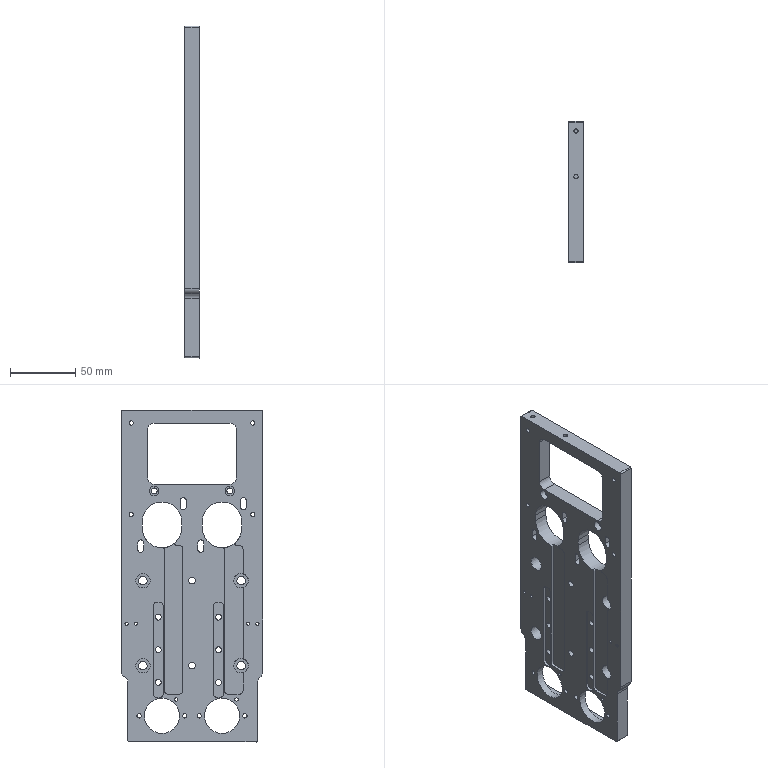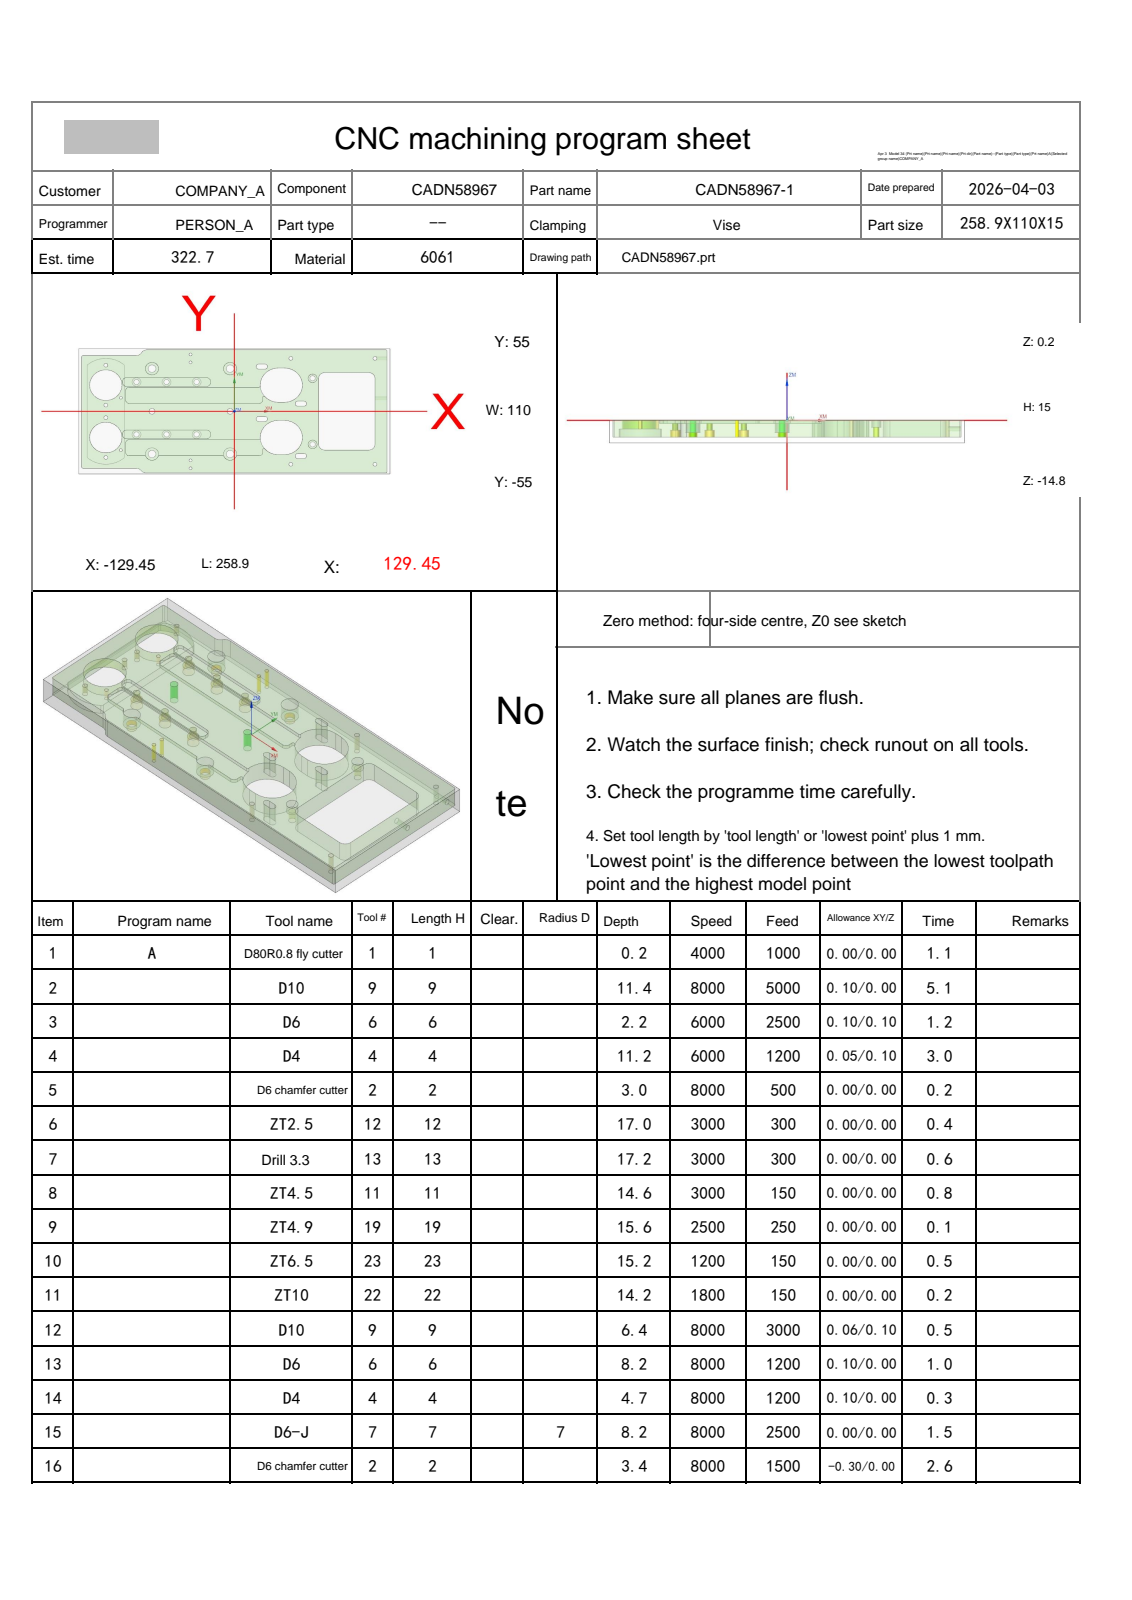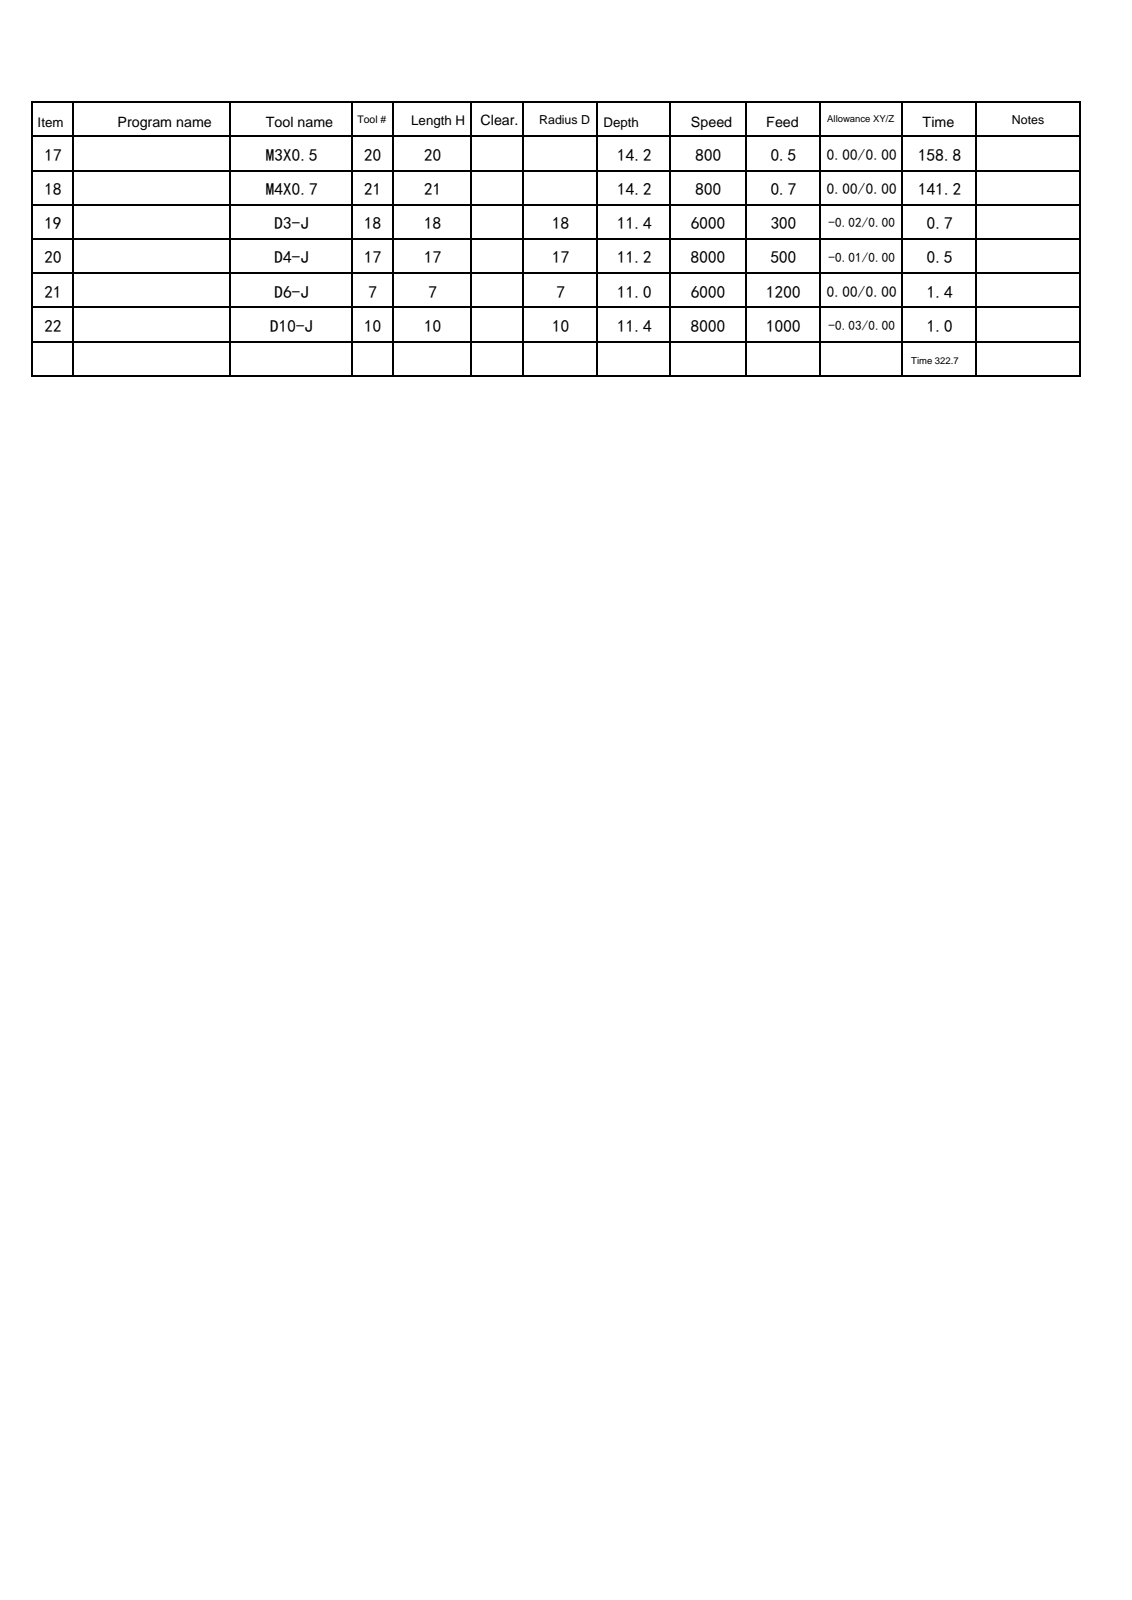NC program | NX | posted by the shop | part box 11 x 108 x 253.9 mm
Lines 911 to 1909 of 8037:
N4 T04 M06
(D4  D=4. R=0. H=04 ce=0.05 di=0.10)
G00 G90 G54 X22.813 Y39.463 M03 S6000
G43 H04 Z20.
M08
Z.5
G01 X20.313 Z.467 F1200.
G03 X20.113 Y39.263 Z.463 I0.0 J-.2
X20.313 Y39.063 Z.458 I.2 J0.0
G01 X25.313 Z.392
X25.376 Z.391
X25.434 Y39.091
X25.472 Y39.141 Z.39
X25.504 Y39.174 Z.389
X25.518 Y39.218
X25.513 Y39.263 Z.388
G03 X25.313 Y39.463 Z.384 I-.2 J0.0
G01 X20.313 Z.317
G03 X20.113 Y39.263 Z.313 I0.0 J-.2
X20.313 Y39.063 Z.309 I.2 J0.0
G01 X25.313 Z.243
X25.376 Z.242
X25.434 Y39.091 Z.241
X25.472 Y39.141 Z.24
X25.504 Y39.174
X25.518 Y39.218 Z.239
X25.513 Y39.263
G03 X25.313 Y39.463 Z.234 I-.2 J0.0
G01 X20.313 Z.168
G03 X20.113 Y39.263 Z.164 I0.0 J-.2
X20.313 Y39.063 Z.16 I.2 J0.0
G01 X25.313 Z.093
X25.376
X25.434 Y39.091 Z.092
X25.472 Y39.141 Z.091
X25.504 Y39.174 Z.09
X25.518 Y39.218
X25.513 Y39.263 Z.089
G03 X25.313 Y39.463 Z.085 I-.2 J0.0
G01 X20.313 Z.019
G03 X20.113 Y39.263 Z.015 I0.0 J-.2
X20.313 Y39.063 Z.01 I.2 J0.0
G01 X25.313 Z-.056
X25.376 Z-.057
X25.434 Y39.091 Z-.058
X25.472 Y39.141
X25.504 Y39.174 Z-.059
X25.518 Y39.218
X25.513 Y39.263 Z-.06
G03 X25.313 Y39.463 Z-.064 I-.2 J0.0
G01 X20.313 Z-.131
G03 X20.113 Y39.263 Z-.135 I0.0 J-.2
X20.313 Y39.063 Z-.139 I.2 J0.0
G01 X25.313 Z-.205
X25.376 Z-.206
X25.434 Y39.091 Z-.207
X25.472 Y39.141 Z-.208
X25.504 Y39.174
X25.518 Y39.218 Z-.209
X25.513 Y39.263
G03 X25.313 Y39.463 Z-.214 I-.2 J0.0
G01 X20.313 Z-.28
G03 X20.113 Y39.263 Z-.284 I0.0 J-.2
X20.313 Y39.063 Z-.288 I.2 J0.0
G01 X25.313 Z-.355
X25.376
X25.434 Y39.091 Z-.356
X25.472 Y39.141 Z-.357
X25.504 Y39.174 Z-.358
X25.518 Y39.218
X25.513 Y39.263 Z-.359
G03 X25.313 Y39.463 Z-.363 I-.2 J0.0
G01 X20.313 Z-.429
G03 X20.113 Y39.263 Z-.433 I0.0 J-.2
X20.313 Y39.063 Z-.438 I.2 J0.0
G01 X25.313 Z-.504
X25.376 Z-.505
X25.434 Y39.091 Z-.506
X25.472 Y39.141
X25.504 Y39.174 Z-.507
X25.518 Y39.218 Z-.508
X25.513 Y39.263
G03 X25.313 Y39.463 Z-.512 I-.2 J0.0
G01 X20.313 Z-.579
G03 X20.113 Y39.263 Z-.583 I0.0 J-.2
X20.313 Y39.063 Z-.587 I.2 J0.0
G01 X25.313 Z-.653
X25.376 Z-.654
X25.434 Y39.091 Z-.655
X25.472 Y39.141 Z-.656
X25.504 Y39.174
X25.518 Y39.218 Z-.657
X25.513 Y39.263
G03 X25.313 Y39.463 Z-.662 I-.2 J0.0
G01 X20.313 Z-.728
G03 X20.113 Y39.263 Z-.732 I0.0 J-.2
X20.313 Y39.063 Z-.736 I.2 J0.0
G01 X25.313 Z-.803
X25.376
X25.434 Y39.091 Z-.804
X25.472 Y39.141 Z-.805
X25.504 Y39.174 Z-.806
X25.518 Y39.218
X25.513 Y39.263 Z-.807
G03 X25.313 Y39.463 Z-.811 I-.2 J0.0
G01 X20.313 Z-.877
G03 X20.113 Y39.263 Z-.881 I0.0 J-.2
X20.313 Y39.063 Z-.886 I.2 J0.0
G01 X25.313 Z-.952
X25.376 Z-.953
X25.434 Y39.091 Z-.954
X25.472 Y39.141
X25.504 Y39.174 Z-.955
X25.518 Y39.218 Z-.956
X25.513 Y39.263
G03 X25.313 Y39.463 Z-.96 I-.2 J0.0
G01 X20.313 Z-1.027
G03 X20.113 Y39.263 Z-1.031 I0.0 J-.2
X20.313 Y39.063 Z-1.035 I.2 J0.0
G01 X25.313 Z-1.101
X25.376 Z-1.102
X25.434 Y39.091 Z-1.103
X25.472 Y39.141 Z-1.104
X25.504 Y39.174
X25.518 Y39.218 Z-1.105
X25.513 Y39.263 Z-1.106
G03 X25.313 Y39.463 Z-1.11 I-.2 J0.0
G01 X20.313 Z-1.176
G03 X20.113 Y39.263 Z-1.18 I0.0 J-.2
X20.313 Y39.063 Z-1.184 I.2 J0.0
G01 X25.313 Z-1.251
X25.376 Z-1.252
X25.434 Y39.091
X25.472 Y39.141 Z-1.253
X25.504 Y39.174 Z-1.254
X25.518 Y39.218
X25.513 Y39.263 Z-1.255
G03 X25.313 Y39.463 Z-1.259 I-.2 J0.0
G01 X20.313 Z-1.325
G03 X20.113 Y39.263 Z-1.33 I0.0 J-.2
X20.313 Y39.063 Z-1.334 I.2 J0.0
G01 X25.313 Z-1.4
X25.376 Z-1.401
X25.434 Y39.091 Z-1.402
X25.472 Y39.141
X25.504 Y39.174 Z-1.403
X25.518 Y39.218 Z-1.404
X25.513 Y39.263
G03 X25.313 Y39.463 Z-1.408 I-.2 J0.0
G01 X20.313 Z-1.475
G03 X20.113 Y39.263 Z-1.479 I0.0 J-.2
X20.313 Y39.063 Z-1.483 I.2 J0.0
G01 X25.313 Z-1.549
X25.376 Z-1.55
X25.434 Y39.091 Z-1.551
X25.472 Y39.141 Z-1.552
X25.504 Y39.174
X25.518 Y39.218 Z-1.553
X25.513 Y39.263 Z-1.554
G03 X25.313 Y39.463 Z-1.558 I-.2 J0.0
G01 X20.313 Z-1.624
G03 X20.113 Y39.263 Z-1.628 I0.0 J-.2
X20.313 Y39.063 Z-1.632 I.2 J0.0
G01 X25.313 Z-1.699
X25.376 Z-1.7
X25.434 Y39.091
X25.472 Y39.141 Z-1.701
X25.504 Y39.174 Z-1.702
X25.518 Y39.218
X25.513 Y39.263 Z-1.703
G03 X25.313 Y39.463 Z-1.707 I-.2 J0.0
G01 X20.313 Z-1.773
G03 X20.113 Y39.263 Z-1.778 I0.0 J-.2
X20.313 Y39.063 Z-1.782 I.2 J0.0
G01 X25.313 Z-1.848
X25.376 Z-1.849
X25.434 Y39.091 Z-1.85
X25.472 Y39.141 Z-1.851
X25.504 Y39.174
X25.518 Y39.218 Z-1.852
X25.513 Y39.263
G03 X25.313 Y39.463 Z-1.856 I-.2 J0.0
G01 X20.313 Z-1.923
G03 X20.113 Y39.263 Z-1.927 I0.0 J-.2
X20.313 Y39.063 Z-1.931 I.2 J0.0
G01 X25.313 Z-1.997
X25.376 Z-1.998
X25.434 Y39.091 Z-1.999
X25.472 Y39.141 Z-2.
X25.504 Y39.174
X25.518 Y39.218 Z-2.001
X25.513 Y39.263 Z-2.002
G03 X25.313 Y39.463 Z-2.006 I-.2 J0.0
G01 X20.313 Z-2.072
G03 X20.113 Y39.263 Z-2.076 I0.0 J-.2
X20.313 Y39.063 Z-2.08 I.2 J0.0
G01 X25.313 Z-2.147
X25.376 Z-2.148
X25.434 Y39.091
X25.472 Y39.141 Z-2.149
X25.504 Y39.174 Z-2.15
X25.518 Y39.218
X25.513 Y39.263 Z-2.151
G03 X25.313 Y39.463 Z-2.155 I-.2 J0.0
G01 X20.313 Z-2.221
G03 X20.113 Y39.263 Z-2.226 I0.0 J-.2
X20.313 Y39.063 Z-2.23 I.2 J0.0
G01 X25.313 Z-2.296
X25.376 Z-2.297
X25.434 Y39.091 Z-2.298
X25.472 Y39.141 Z-2.299
X25.504 Y39.174
X25.518 Y39.218 Z-2.3
X25.513 Y39.263
G03 X25.313 Y39.463 Z-2.304 I-.2 J0.0
G01 X20.313 Z-2.371
G03 X20.113 Y39.263 Z-2.375 I0.0 J-.2
X20.313 Y39.063 Z-2.379 I.2 J0.0
G01 X25.313 Z-2.446
X25.376
X25.434 Y39.091 Z-2.447
X25.472 Y39.141 Z-2.448
X25.504 Y39.174 Z-2.449
X25.518 Y39.218
X25.513 Y39.263 Z-2.45
G03 X25.313 Y39.463 Z-2.454 I-.2 J0.0
G01 X20.313 Z-2.52
G03 X20.113 Y39.263 Z-2.524 I0.0 J-.2
X20.313 Y39.063 Z-2.529 I.2 J0.0
G01 X25.313 Z-2.595
X25.376 Z-2.596
X25.434 Y39.091
X25.472 Y39.141 Z-2.597
X25.504 Y39.174 Z-2.598
X25.518 Y39.218
X25.513 Y39.263 Z-2.599
G03 X25.313 Y39.463 Z-2.603 I-.2 J0.0
G01 X20.313 Z-2.67
G03 X20.113 Y39.263 Z-2.674 I0.0 J-.2
X20.313 Y39.063 Z-2.678 I.2 J0.0
G01 X25.313 Z-2.744
X25.376 Z-2.745
X25.434 Y39.091 Z-2.746
X25.472 Y39.141 Z-2.747
X25.504 Y39.174
X25.518 Y39.218 Z-2.748
X25.513 Y39.263
G03 X25.313 Y39.463 Z-2.753 I-.2 J0.0
G01 X20.313 Z-2.819
G03 X20.113 Y39.263 Z-2.823 I0.0 J-.2
X20.313 Y39.063 Z-2.827 I.2 J0.0
G01 X25.313 Z-2.894
X25.376
X25.434 Y39.091 Z-2.895
X25.472 Y39.141 Z-2.896
X25.504 Y39.174 Z-2.897
X25.518 Y39.218
X25.513 Y39.263 Z-2.898
G03 X25.313 Y39.463 Z-2.902 I-.2 J0.0
G01 X20.313 Z-2.968
G03 X20.113 Y39.263 Z-2.972 I0.0 J-.2
X20.313 Y39.063 Z-2.977 I.2 J0.0
G01 X25.313 Z-3.043
X25.376 Z-3.044
X25.434 Y39.091 Z-3.045
X25.472 Y39.141
X25.504 Y39.174 Z-3.046
X25.518 Y39.218
X25.513 Y39.263 Z-3.047
G03 X25.313 Y39.463 Z-3.051 I-.2 J0.0
G01 X20.313 Z-3.118
G03 X20.113 Y39.263 Z-3.122 I0.0 J-.2
X20.313 Y39.063 Z-3.126 I.2 J0.0
G01 X25.313 Z-3.192
X25.376 Z-3.193
X25.434 Y39.091 Z-3.194
X25.472 Y39.141 Z-3.195
X25.504 Y39.174
X25.518 Y39.218 Z-3.196
X25.513 Y39.263
G03 X25.313 Y39.463 Z-3.201 I-.2 J0.0
G01 X20.313 Z-3.267
G03 X20.113 Y39.263 Z-3.271 I0.0 J-.2
X20.313 Y39.063 Z-3.275 I.2 J0.0
G01 X25.313 Z-3.342
X25.376
X25.434 Y39.091 Z-3.343
X25.472 Y39.141 Z-3.344
X25.504 Y39.174 Z-3.345
X25.518 Y39.218
X25.513 Y39.263 Z-3.346
G03 X25.313 Y39.463 Z-3.35 I-.2 J0.0
G01 X20.313 Z-3.416
G03 X20.113 Y39.263 Z-3.42 I0.0 J-.2
X20.313 Y39.063 Z-3.425 I.2 J0.0
G01 X25.313 Z-3.491
X25.376 Z-3.492
X25.434 Y39.091 Z-3.493
X25.472 Y39.141
X25.504 Y39.174 Z-3.494
X25.518 Y39.218 Z-3.495
X25.513 Y39.263
G03 X25.313 Y39.463 Z-3.499 I-.2 J0.0
G01 X20.313 Z-3.566
G03 X20.113 Y39.263 Z-3.57 I0.0 J-.2
X20.313 Y39.063 Z-3.574 I.2 J0.0
G01 X25.313 Z-3.64
X25.376 Z-3.641
X25.434 Y39.091 Z-3.642
X25.472 Y39.141 Z-3.643
X25.504 Y39.174
X25.518 Y39.218 Z-3.644
X25.513 Y39.263
G03 X25.313 Y39.463 Z-3.649 I-.2 J0.0
G01 X20.313 Z-3.715
G03 X20.113 Y39.263 Z-3.719 I0.0 J-.2
X20.313 Y39.063 Z-3.723 I.2 J0.0
G01 X25.313 Z-3.79
X25.376
X25.434 Y39.091 Z-3.791
X25.472 Y39.141 Z-3.792
X25.504 Y39.174 Z-3.793
X25.518 Y39.218
X25.513 Y39.263 Z-3.794
G03 X25.313 Y39.463 Z-3.798 I-.2 J0.0
G01 X20.313 Z-3.864
G03 X20.113 Y39.263 Z-3.869 I0.0 J-.2
X20.313 Y39.063 Z-3.873 I.2 J0.0
G01 X25.313 Z-3.939
X25.376 Z-3.94
X25.434 Y39.091 Z-3.941
X25.472 Y39.141
X25.504 Y39.174 Z-3.942
X25.518 Y39.218 Z-3.943
X25.513 Y39.263
G03 X25.313 Y39.463 Z-3.947 I-.2 J0.0
G01 X20.313 Z-4.014
G03 X20.113 Y39.263 Z-4.018 I0.0 J-.2
X20.313 Y39.063 Z-4.022 I.2 J0.0
G01 X25.313 Z-4.088
X25.376 Z-4.089
X25.434 Y39.091 Z-4.09
X25.472 Y39.141 Z-4.091
X25.504 Y39.174
X25.518 Y39.218 Z-4.092
X25.513 Y39.263 Z-4.093
G03 X25.313 Y39.463 Z-4.097 I-.2 J0.0
G01 X20.313 Z-4.163
G03 X20.113 Y39.263 Z-4.167 I0.0 J-.2
X20.313 Y39.063 Z-4.171 I.2 J0.0
G01 X25.313 Z-4.238
X25.376 Z-4.239
X25.434 Y39.091
X25.472 Y39.141 Z-4.24
X25.504 Y39.174 Z-4.241
X25.518 Y39.218
X25.513 Y39.263 Z-4.242
G03 X25.313 Y39.463 Z-4.246 I-.2 J0.0
G01 X20.313 Z-4.312
G03 X20.113 Y39.263 Z-4.317 I0.0 J-.2
X20.313 Y39.063 Z-4.321 I.2 J0.0
G01 X25.313 Z-4.387
X25.376 Z-4.388
X25.434 Y39.091 Z-4.389
X25.472 Y39.141
X25.504 Y39.174 Z-4.39
X25.518 Y39.218 Z-4.391
X25.513 Y39.263
G03 X25.313 Y39.463 Z-4.395 I-.2 J0.0
G01 X20.313 Z-4.462
G03 X20.113 Y39.263 Z-4.466 I0.0 J-.2
X20.313 Y39.063 Z-4.47 I.2 J0.0
G01 X25.313 Z-4.536
X25.376 Z-4.537
X25.434 Y39.091 Z-4.538
X25.472 Y39.141 Z-4.539
X25.504 Y39.174
X25.518 Y39.218 Z-4.54
X25.513 Y39.263 Z-4.541
G03 X25.313 Y39.463 Z-4.545 I-.2 J0.0
G01 X20.313 Z-4.611
G03 X20.113 Y39.263 Z-4.615 I0.0 J-.2
X20.313 Y39.063 Z-4.619 I.2 J0.0
G01 X25.313 Z-4.686
X25.376 Z-4.687
X25.434 Y39.091
X25.472 Y39.141 Z-4.688
X25.504 Y39.174 Z-4.689
X25.518 Y39.218
X25.513 Y39.263 Z-4.69
G03 X25.313 Y39.463 Z-4.694 I-.2 J0.0
G01 X20.313 Z-4.76
G03 X20.113 Y39.263 Z-4.765 I0.0 J-.2
X20.313 Y39.063 Z-4.769 I.2 J0.0
G01 X25.313 Z-4.835
X25.376 Z-4.836
X25.434 Y39.091 Z-4.837
X25.472 Y39.141 Z-4.838
X25.504 Y39.174
X25.518 Y39.218 Z-4.839
X25.513 Y39.263
G03 X25.313 Y39.463 Z-4.843 I-.2 J0.0
G01 X20.313 Z-4.91
G03 X20.113 Y39.263 Z-4.914 I0.0 J-.2
X20.313 Y39.063 Z-4.918 I.2 J0.0
G01 X25.313 Z-4.984
X25.376 Z-4.985
X25.434 Y39.091 Z-4.986
X25.472 Y39.141 Z-4.987
X25.504 Y39.174
X25.518 Y39.218 Z-4.988
X25.513 Y39.263 Z-4.989
G03 X25.313 Y39.463 Z-4.993 I-.2 J0.0
G01 X20.313 Z-5.059
G03 X20.113 Y39.263 Z-5.063 I0.0 J-.2
X20.313 Y39.063 Z-5.067 I.2 J0.0
G01 X25.313 Z-5.134
X25.376 Z-5.135
X25.434 Y39.091
X25.472 Y39.141 Z-5.136
X25.504 Y39.174 Z-5.137
X25.518 Y39.218
X25.513 Y39.263 Z-5.138
G03 X25.313 Y39.463 Z-5.142 I-.2 J0.0
G01 X20.313 Z-5.208
G03 X20.113 Y39.263 Z-5.213 I0.0 J-.2
X20.313 Y39.063 Z-5.217 I.2 J0.0
G01 X25.313 Z-5.283
X25.376 Z-5.284
X25.434 Y39.091 Z-5.285
X25.472 Y39.141 Z-5.286
X25.504 Y39.174
X25.518 Y39.218 Z-5.287
X25.513 Y39.263
G03 X25.313 Y39.463 Z-5.292 I-.2 J0.0
G01 X20.313 Z-5.358
G03 X20.113 Y39.263 Z-5.362 I0.0 J-.2
X20.313 Y39.063 Z-5.366 I.2 J0.0
G01 X25.313 Z-5.433
X25.376
X25.434 Y39.091 Z-5.434
X25.472 Y39.141 Z-5.435
X25.504 Y39.174 Z-5.436
X25.518 Y39.218
X25.513 Y39.263 Z-5.437
G03 X25.313 Y39.463 Z-5.441 I-.2 J0.0
G01 X20.313 Z-5.507
G03 X20.113 Y39.263 Z-5.511 I0.0 J-.2
X20.313 Y39.063 Z-5.516 I.2 J0.0
G01 X25.313 Z-5.582
X25.376 Z-5.583
X25.434 Y39.091
X25.472 Y39.141 Z-5.584
X25.504 Y39.174 Z-5.585
X25.518 Y39.218
X25.513 Y39.263 Z-5.586
G03 X25.313 Y39.463 Z-5.59 I-.2 J0.0
G01 X20.313 Z-5.657
G03 X20.113 Y39.263 Z-5.661 I0.0 J-.2
X20.313 Y39.063 Z-5.665 I.2 J0.0
G01 X25.313 Z-5.731
X25.376 Z-5.732
X25.434 Y39.091 Z-5.733
X25.472 Y39.141 Z-5.734
X25.504 Y39.174
X25.518 Y39.218 Z-5.735
X25.513 Y39.263
G03 X25.313 Y39.463 Z-5.74 I-.2 J0.0
G01 X20.313 Z-5.806
G03 X20.113 Y39.263 Z-5.81 I0.0 J-.2
X20.313 Y39.063 Z-5.814 I.2 J0.0
G01 X25.313 Z-5.881
X25.376
X25.434 Y39.091 Z-5.882
X25.472 Y39.141 Z-5.883
X25.504 Y39.174 Z-5.884
X25.518 Y39.218
X25.513 Y39.263 Z-5.885
G03 X25.313 Y39.463 Z-5.889 I-.2 J0.0
G01 X20.313 Z-5.955
G03 X20.113 Y39.263 Z-5.959 I0.0 J-.2
X20.313 Y39.063 Z-5.964 I.2 J0.0
G01 X25.313 Z-6.03
X25.376 Z-6.031
X25.434 Y39.091 Z-6.032
X25.472 Y39.141
X25.504 Y39.174 Z-6.033
X25.518 Y39.218 Z-6.034
X25.513 Y39.263
G03 X25.313 Y39.463 Z-6.038 I-.2 J0.0
G01 X20.313 Z-6.105
G03 X20.113 Y39.263 Z-6.109 I0.0 J-.2
X20.313 Y39.063 Z-6.113 I.2 J0.0
G01 X25.313 Z-6.179
X25.376 Z-6.18
X25.434 Y39.091 Z-6.181
X25.472 Y39.141 Z-6.182
X25.504 Y39.174
X25.518 Y39.218 Z-6.183
X25.513 Y39.263
G03 X25.313 Y39.463 Z-6.188 I-.2 J0.0
G01 X20.313 Z-6.254
G03 X20.113 Y39.263 Z-6.258 I0.0 J-.2
X20.313 Y39.063 Z-6.262 I.2 J0.0
G01 X25.313 Z-6.329
X25.376
X25.434 Y39.091 Z-6.33
X25.472 Y39.141 Z-6.331
X25.504 Y39.174 Z-6.332
X25.518 Y39.218
X25.513 Y39.263 Z-6.333
G03 X25.313 Y39.463 Z-6.337 I-.2 J0.0
G01 X20.313 Z-6.403
G03 X20.113 Y39.263 Z-6.407 I0.0 J-.2
X20.313 Y39.063 Z-6.412 I.2 J0.0
G01 X25.313 Z-6.478
X25.376 Z-6.479
X25.434 Y39.091 Z-6.48
X25.472 Y39.141
X25.504 Y39.174 Z-6.481
X25.518 Y39.218 Z-6.482
X25.513 Y39.263
G03 X25.313 Y39.463 Z-6.486 I-.2 J0.0
G01 X20.313 Z-6.553
G03 X20.113 Y39.263 Z-6.557 I0.0 J-.2
X20.313 Y39.063 Z-6.561 I.2 J0.0
G01 X25.313 Z-6.627
X25.376 Z-6.628
X25.434 Y39.091 Z-6.629
X25.472 Y39.141 Z-6.63
X25.504 Y39.174
X25.518 Y39.218 Z-6.631
X25.513 Y39.263
G03 X25.313 Y39.463 Z-6.636 I-.2 J0.0
G01 X20.313 Z-6.702
G03 X20.113 Y39.263 Z-6.706 I0.0 J-.2
X20.313 Y39.063 Z-6.71 I.2 J0.0
G01 X25.313 Z-6.777
X25.376
X25.434 Y39.091 Z-6.778
X25.472 Y39.141 Z-6.779
X25.504 Y39.174 Z-6.78
X25.518 Y39.218
X25.513 Y39.263 Z-6.781
G03 X25.313 Y39.463 Z-6.785 I-.2 J0.0
G01 X20.313 Z-6.851
G03 X20.113 Y39.263 Z-6.856 I0.0 J-.2
X20.313 Y39.063 Z-6.86 I.2 J0.0
G01 X25.313 Z-6.926
X25.376 Z-6.927
X25.434 Y39.091 Z-6.928
X25.472 Y39.141
X25.504 Y39.174 Z-6.929
X25.518 Y39.218 Z-6.93
X25.513 Y39.263
G03 X25.313 Y39.463 Z-6.934 I-.2 J0.0
G01 X20.313 Z-7.001
G03 X20.113 Y39.263 Z-7.005 I0.0 J-.2
X20.313 Y39.063 Z-7.009 I.2 J0.0
G01 X25.313 Z-7.075
X25.376 Z-7.076
X25.434 Y39.091 Z-7.077
X25.472 Y39.141 Z-7.078
X25.504 Y39.174
X25.518 Y39.218 Z-7.079
X25.513 Y39.263 Z-7.08
G03 X25.313 Y39.463 Z-7.084 I-.2 J0.0
G01 X20.313 Z-7.15
G03 X20.113 Y39.263 Z-7.154 I0.0 J-.2
X20.313 Y39.063 Z-7.158 I.2 J0.0
G01 X25.313 Z-7.225
X25.376 Z-7.226
X25.434 Y39.091
X25.472 Y39.141 Z-7.227
X25.504 Y39.174 Z-7.228
X25.518 Y39.218
X25.513 Y39.263 Z-7.229
G03 X25.313 Y39.463 Z-7.233 I-.2 J0.0
G01 X20.313 Z-7.299
G03 X20.113 Y39.263 Z-7.304 I0.0 J-.2
X20.313 Y39.063 Z-7.308 I.2 J0.0
G01 X25.313 Z-7.374
X25.376 Z-7.375
X25.434 Y39.091 Z-7.376
X25.472 Y39.141 Z-7.377
X25.504 Y39.174
X25.518 Y39.218 Z-7.378
X25.513 Y39.263
G03 X25.313 Y39.463 Z-7.382 I-.2 J0.0
G01 X20.313 Z-7.449
G03 X20.113 Y39.263 Z-7.453 I0.0 J-.2
X20.313 Y39.063 Z-7.457 I.2 J0.0
G01 X25.313 Z-7.523
X25.376 Z-7.524
X25.434 Y39.091 Z-7.525
X25.472 Y39.141 Z-7.526
X25.504 Y39.174
X25.518 Y39.218 Z-7.527
X25.513 Y39.263 Z-7.528
G03 X25.313 Y39.463 Z-7.532 I-.2 J0.0
G01 X20.313 Z-7.598
G03 X20.113 Y39.263 Z-7.602 I0.0 J-.2
X20.313 Y39.063 Z-7.606 I.2 J0.0
G01 X25.313 Z-7.673
X25.376 Z-7.674
X25.434 Y39.091
X25.472 Y39.141 Z-7.675
X25.504 Y39.174 Z-7.676
X25.518 Y39.218
X25.513 Y39.263 Z-7.677
G03 X25.313 Y39.463 Z-7.681 I-.2 J0.0
G01 X20.313 Z-7.747
G03 X20.113 Y39.263 Z-7.752 I0.0 J-.2
X20.313 Y39.063 Z-7.756 I.2 J0.0
G01 X25.313 Z-7.822
X25.376 Z-7.823
X25.434 Y39.091 Z-7.824
X25.472 Y39.141 Z-7.825
X25.504 Y39.174
X25.518 Y39.218 Z-7.826
X25.513 Y39.263
G03 X25.313 Y39.463 Z-7.83 I-.2 J0.0
G01 X20.313 Z-7.897
G03 X20.113 Y39.263 Z-7.901 I0.0 J-.2
X20.313 Y39.063 Z-7.905 I.2 J0.0
G01 X25.313 Z-7.971
X25.376 Z-7.972
X25.434 Y39.091 Z-7.973
X25.472 Y39.141 Z-7.974
X25.504 Y39.174
X25.518 Y39.218 Z-7.975
X25.513 Y39.263 Z-7.976
G03 X25.313 Y39.463 Z-7.98 I-.2 J0.0
G01 X20.313 Z-8.046
G03 X20.113 Y39.263 Z-8.05 I0.0 J-.2
X20.313 Y39.063 Z-8.054 I.2 J0.0
G01 X25.313 Z-8.121
X25.376 Z-8.122
X25.434 Y39.091
X25.472 Y39.141 Z-8.123
X25.504 Y39.174 Z-8.124
X25.518 Y39.218
X25.513 Y39.263 Z-8.125
G03 X25.313 Y39.463 Z-8.129 I-.2 J0.0
G01 X20.313 Z-8.196
G03 X20.113 Y39.263 Z-8.2 I0.0 J-.2
X20.313 Y39.063 Z-8.204 I.2 J0.0
G01 X25.313 Z-8.27
X25.376 Z-8.271
X25.434 Y39.091 Z-8.272
X25.472 Y39.141 Z-8.273
X25.504 Y39.174
X25.518 Y39.218 Z-8.274
X25.513 Y39.263
G03 X25.313 Y39.463 Z-8.279 I-.2 J0.0
G01 X20.313 Z-8.345
G03 X20.113 Y39.263 Z-8.349 I0.0 J-.2
X20.313 Y39.063 Z-8.353 I.2 J0.0
G01 X25.313 Z-8.42
X25.376
X25.434 Y39.091 Z-8.421
X25.472 Y39.141 Z-8.422
X25.504 Y39.174 Z-8.423
X25.518 Y39.218
X25.513 Y39.263 Z-8.424
G03 X25.313 Y39.463 Z-8.428 I-.2 J0.0
G01 X20.313 Z-8.494
G03 X20.113 Y39.263 Z-8.498 I0.0 J-.2
X20.313 Y39.063 Z-8.503 I.2 J0.0
G01 X25.313 Z-8.569
X25.376 Z-8.57
X25.434 Y39.091 Z-8.571
X25.472 Y39.141
X25.504 Y39.174 Z-8.572
X25.518 Y39.218
X25.513 Y39.263 Z-8.573
G03 X25.313 Y39.463 Z-8.577 I-.2 J0.0
G01 X20.313 Z-8.644
G03 X20.113 Y39.263 Z-8.648 I0.0 J-.2
X20.313 Y39.063 Z-8.652 I.2 J0.0
G01 X25.313 Z-8.718
X25.376 Z-8.719
X25.434 Y39.091 Z-8.72
X25.472 Y39.141 Z-8.721
X25.504 Y39.174
X25.518 Y39.218 Z-8.722
X25.513 Y39.263
G03 X25.313 Y39.463 Z-8.727 I-.2 J0.0
G01 X20.313 Z-8.793
G03 X20.113 Y39.263 Z-8.797 I0.0 J-.2
X20.313 Y39.063 Z-8.801 I.2 J0.0
G01 X25.313 Z-8.868
X25.376
X25.434 Y39.091 Z-8.869
X25.472 Y39.141 Z-8.87
X25.504 Y39.174 Z-8.871
X25.518 Y39.218
X25.513 Y39.263 Z-8.872
G03 X25.313 Y39.463 Z-8.876 I-.2 J0.0
G01 X20.313 Z-8.942
G03 X20.113 Y39.263 Z-8.946 I0.0 J-.2
X20.313 Y39.063 Z-8.951 I.2 J0.0
G01 X25.313 Z-9.017
X25.376 Z-9.018
X25.434 Y39.091 Z-9.019
X25.472 Y39.141
X25.504 Y39.174 Z-9.02
X25.518 Y39.218 Z-9.021
X25.513 Y39.263
G03 X25.313 Y39.463 Z-9.025 I-.2 J0.0
G01 X20.313 Z-9.092
G03 X20.113 Y39.263 Z-9.096 I0.0 J-.2
X20.313 Y39.063 Z-9.1 I.2 J0.0
G01 X25.313 Z-9.166
X25.376 Z-9.167
X25.434 Y39.091 Z-9.168
X25.472 Y39.141 Z-9.169
X25.504 Y39.174
X25.518 Y39.218 Z-9.17
X25.513 Y39.263
G03 X25.313 Y39.463 Z-9.175 I-.2 J0.0
G01 X20.313 Z-9.241
G03 X20.113 Y39.263 Z-9.245 I0.0 J-.2
X20.313 Y39.063 Z-9.249 I.2 J0.0
G01 X25.313 Z-9.316
X25.376
X25.434 Y39.091 Z-9.317
X25.472 Y39.141 Z-9.318
X25.504 Y39.174 Z-9.319
X25.518 Y39.218
X25.513 Y39.263 Z-9.32
G03 X25.313 Y39.463 Z-9.324 I-.2 J0.0
G01 X20.313 Z-9.39
G03 X20.113 Y39.263 Z-9.394 I0.0 J-.2
X20.313 Y39.063 Z-9.399 I.2 J0.0
G01 X25.313 Z-9.465
X25.376 Z-9.466
X25.434 Y39.091 Z-9.467
X25.472 Y39.141
X25.504 Y39.174 Z-9.468
X25.518 Y39.218 Z-9.469
X25.513 Y39.263
G03 X25.313 Y39.463 Z-9.473 I-.2 J0.0
G01 X20.313 Z-9.54
G03 X20.113 Y39.263 Z-9.544 I0.0 J-.2
X20.313 Y39.063 Z-9.548 I.2 J0.0
G01 X25.313 Z-9.614
X25.376 Z-9.615
X25.434 Y39.091 Z-9.616
X25.472 Y39.141 Z-9.617
X25.504 Y39.174
X25.518 Y39.218 Z-9.618
X25.513 Y39.263 Z-9.619
G03 X25.313 Y39.463 Z-9.623 I-.2 J0.0
G01 X20.313 Z-9.689
G03 X20.113 Y39.263 Z-9.693 I0.0 J-.2
X20.313 Y39.063 Z-9.697 I.2 J0.0
G01 X25.313 Z-9.764
X25.376
X25.434 Y39.091 Z-9.765
X25.472 Y39.141 Z-9.766
X25.504 Y39.174 Z-9.767
X25.518 Y39.218
X25.513 Y39.263 Z-9.768
G03 X25.313 Y39.463 Z-9.772 I-.2 J0.0
G01 X20.313 Z-9.838
G03 X20.113 Y39.263 Z-9.843 I0.0 J-.2
X20.313 Y39.063 Z-9.847 I.2 J0.0
G01 X25.313 Z-9.913
X25.376 Z-9.914
X25.434 Y39.091 Z-9.915
X25.472 Y39.141
X25.504 Y39.174 Z-9.916
X25.518 Y39.218 Z-9.917
X25.513 Y39.263
G03 X25.313 Y39.463 Z-9.921 I-.2 J0.0
G01 X20.313 Z-9.988
G03 X20.113 Y39.263 Z-9.992 I0.0 J-.2
X20.313 Y39.063 Z-9.996 I.2 J0.0
G01 X25.313 Z-10.062
X25.376 Z-10.063
X25.434 Y39.091 Z-10.064
X25.472 Y39.141 Z-10.065
X25.504 Y39.174
X25.518 Y39.218 Z-10.066
X25.513 Y39.263 Z-10.067
G03 X25.313 Y39.463 Z-10.071 I-.2 J0.0
G01 X20.313 Z-10.137
G03 X20.113 Y39.263 Z-10.141 I0.0 J-.2
X20.313 Y39.063 Z-10.145 I.2 J0.0
G01 X25.313 Z-10.212
X25.376 Z-10.213
X25.434 Y39.091
X25.472 Y39.141 Z-10.214
X25.504 Y39.174 Z-10.215
X25.518 Y39.218
X25.513 Y39.263 Z-10.216
G03 X25.313 Y39.463 Z-10.22 I-.2 J0.0
G01 X20.313 Z-10.286
G03 X20.113 Y39.263 Z-10.291 I0.0 J-.2
X20.313 Y39.063 Z-10.295 I.2 J0.0
G01 X25.313 Z-10.361
X25.376 Z-10.362
X25.434 Y39.091 Z-10.363
X25.472 Y39.141 Z-10.364
X25.504 Y39.174
X25.518 Y39.218 Z-10.365
X25.513 Y39.263
G03 X25.313 Y39.463 Z-10.369 I-.2 J0.0
G01 X20.313 Z-10.436
G03 X20.113 Y39.263 Z-10.44 I0.0 J-.2
X20.313 Y39.063 Z-10.444 I.2 J0.0
G01 X25.313 Z-10.51
X25.376 Z-10.511
X25.434 Y39.091 Z-10.512
X25.472 Y39.141 Z-10.513
X25.504 Y39.174
X25.518 Y39.218 Z-10.514
X25.513 Y39.263 Z-10.515
G03 X25.313 Y39.463 Z-10.519 I-.2 J0.0
G01 X20.313 Z-10.585
G03 X20.113 Y39.263 Z-10.589 I0.0 J-.2
X20.313 Y39.063 Z-10.593 I.2 J0.0
G01 X25.313 Z-10.66
X25.376 Z-10.661
X25.434 Y39.091
X25.472 Y39.141 Z-10.662
X25.504 Y39.174 Z-10.663
X25.518 Y39.218
X25.513 Y39.263 Z-10.664
G03 X25.313 Y39.463 Z-10.668 I-.2 J0.0
G01 X20.313 Z-10.734
G03 X20.113 Y39.263 Z-10.739 I0.0 J-.2
X20.313 Y39.063 Z-10.743 I.2 J0.0
G01 X25.313 Z-10.809
X25.376 Z-10.81
X25.434 Y39.091 Z-10.811
X25.472 Y39.141 Z-10.812
X25.504 Y39.174
X25.518 Y39.218 Z-10.813
X25.513 Y39.263
G03 X25.313 Y39.463 Z-10.817 I-.2 J0.0
G01 X20.313 Z-10.884
G03 X20.113 Y39.263 Z-10.888 I0.0 J-.2
X20.313 Y39.063 Z-10.892 I.2 J0.0
G01 X25.313 Z-10.958
X25.376 Z-10.959
X25.434 Y39.091 Z-10.96
X25.472 Y39.141 Z-10.961
X25.504 Y39.174 Z-10.962
X25.518 Y39.218
X25.513 Y39.263 Z-10.963
G03 X25.313 Y39.463 Z-10.967 I-.2 J0.0
G01 X22.813 Z-11.
X20.313
G03 X20.113 Y39.263 I0.0 J-.2
X20.313 Y39.063 I.2 J0.0
G01 X25.313
G03 X25.513 Y39.263 I0.0 J.2
X25.313 Y39.463 I-.2 J0.0
G01 X22.813
X22.313
Z-10.
G00 Z20.
X55.287 Y6.937
Z.5
G01 X52.787 Z.467
G03 X52.587 Y6.737 Z.463 I0.0 J-.2
X52.787 Y6.537 Z.458 I.2 J0.0
G01 X57.787 Z.392
G03 X57.987 Y6.737 Z.388 I0.0 J.2
G01 Y6.8 Z.387
X57.959 Y6.857 Z.386
X57.909 Y6.895
X57.876 Y6.927 Z.385
X57.832 Y6.942 Z.384
X57.787 Y6.937
X52.787 Z.317
G03 X52.587 Y6.737 Z.313 I0.0 J-.2
X52.787 Y6.537 Z.309 I.2 J0.0
G01 X57.787 Z.243
G03 X57.987 Y6.737 Z.239 I0.0 J.2
G01 Y6.8 Z.238
X57.959 Y6.857 Z.237
X57.909 Y6.895 Z.236
X57.876 Y6.927
X57.832 Y6.942 Z.235
X57.787 Y6.937 Z.234
X52.787 Z.168
G03 X52.587 Y6.737 Z.164 I0.0 J-.2
X52.787 Y6.537 Z.16 I.2 J0.0
G01 X57.787 Z.093
G03 X57.987 Y6.737 Z.089 I0.0 J.2
G01 Y6.8 Z.088
X57.959 Y6.857
X57.909 Y6.895 Z.087
X57.876 Y6.927 Z.086
X57.832 Y6.942
X57.787 Y6.937 Z.085
X52.787 Z.019
G03 X52.587 Y6.737 Z.015 I0.0 J-.2
X52.787 Y6.537 Z.01 I.2 J0.0
G01 X57.787 Z-.056
G03 X57.987 Y6.737 Z-.06 I0.0 J.2
G01 Y6.8 Z-.061
X57.959 Y6.857 Z-.062
X57.909 Y6.895
X57.876 Y6.927 Z-.063
X57.832 Y6.942 Z-.064
X57.787 Y6.937
X52.787 Z-.131
G03 X52.587 Y6.737 Z-.135 I0.0 J-.2
X52.787 Y6.537 Z-.139 I.2 J0.0
G01 X57.787 Z-.205
G03 X57.987 Y6.737 Z-.209 I0.0 J.2
G01 Y6.8 Z-.21
X57.959 Y6.857 Z-.211
X57.909 Y6.895 Z-.212
X57.876 Y6.927
X57.832 Y6.942 Z-.213
X57.787 Y6.937 Z-.214
X52.787 Z-.28
G03 X52.587 Y6.737 Z-.284 I0.0 J-.2
X52.787 Y6.537 Z-.288 I.2 J0.0
G01 X57.787 Z-.355
G03 X57.987 Y6.737 Z-.359 I0.0 J.2
G01 Y6.8 Z-.36
X57.959 Y6.857
X57.909 Y6.895 Z-.361
X57.876 Y6.927 Z-.362
X57.832 Y6.942
X57.787 Y6.937 Z-.363
X52.787 Z-.429
G03 X52.587 Y6.737 Z-.433 I0.0 J-.2
X52.787 Y6.537 Z-.438 I.2 J0.0
G01 X57.787 Z-.504
G03 X57.987 Y6.737 Z-.508 I0.0 J.2
G01 Y6.8 Z-.509
X57.959 Y6.857 Z-.51
X57.909 Y6.895 Z-.511
X57.876 Y6.927
X57.832 Y6.942 Z-.512
X57.787 Y6.937
X52.787 Z-.579
G03 X52.587 Y6.737 Z-.583 I0.0 J-.2
X52.787 Y6.537 Z-.587 I.2 J0.0
G01 X57.787 Z-.653
G03 X57.987 Y6.737 Z-.657 I0.0 J.2
G01 Y6.8 Z-.658
X57.959 Y6.857 Z-.659
X57.909 Y6.895 Z-.66
X57.876 Y6.927
X57.832 Y6.942 Z-.661
X57.787 Y6.937 Z-.662
X52.787 Z-.728
G03 X52.587 Y6.737 Z-.732 I0.0 J-.2
X52.787 Y6.537 Z-.736 I.2 J0.0
G01 X57.787 Z-.803
G03 X57.987 Y6.737 Z-.807 I0.0 J.2
G01 Y6.8 Z-.808
X57.959 Y6.857
X57.909 Y6.895 Z-.809
X57.876 Y6.927 Z-.81
X57.832 Y6.942
X57.787 Y6.937 Z-.811
X52.787 Z-.877
G03 X52.587 Y6.737 Z-.881 I0.0 J-.2
X52.787 Y6.537 Z-.886 I.2 J0.0
G01 X57.787 Z-.952
G03 X57.987 Y6.737 Z-.956 I0.0 J.2
G01 Y6.8 Z-.957
X57.959 Y6.857 Z-.958
X57.909 Y6.895 Z-.959
X57.876 Y6.927
X57.832 Y6.942 Z-.96
X57.787 Y6.937
X52.787 Z-1.027
G03 X52.587 Y6.737 Z-1.031 I0.0 J-.2
X52.787 Y6.537 Z-1.035 I.2 J0.0
G01 X57.787 Z-1.101
G03 X57.987 Y6.737 Z-1.106 I0.0 J.2
G01 Y6.8
X57.959 Y6.857 Z-1.107
X57.909 Y6.895 Z-1.108
X57.876 Y6.927 Z-1.109
X57.832 Y6.942
X57.787 Y6.937 Z-1.11
X52.787 Z-1.176
G03 X52.587 Y6.737 Z-1.18 I0.0 J-.2
X52.787 Y6.537 Z-1.184 I.2 J0.0
G01 X57.787 Z-1.251
G03 X57.987 Y6.737 Z-1.255 I0.0 J.2
G01 Y6.8 Z-1.256
X57.959 Y6.857
X57.909 Y6.895 Z-1.257
X57.876 Y6.927 Z-1.258
X57.832 Y6.942
X57.787 Y6.937 Z-1.259
X52.787 Z-1.325